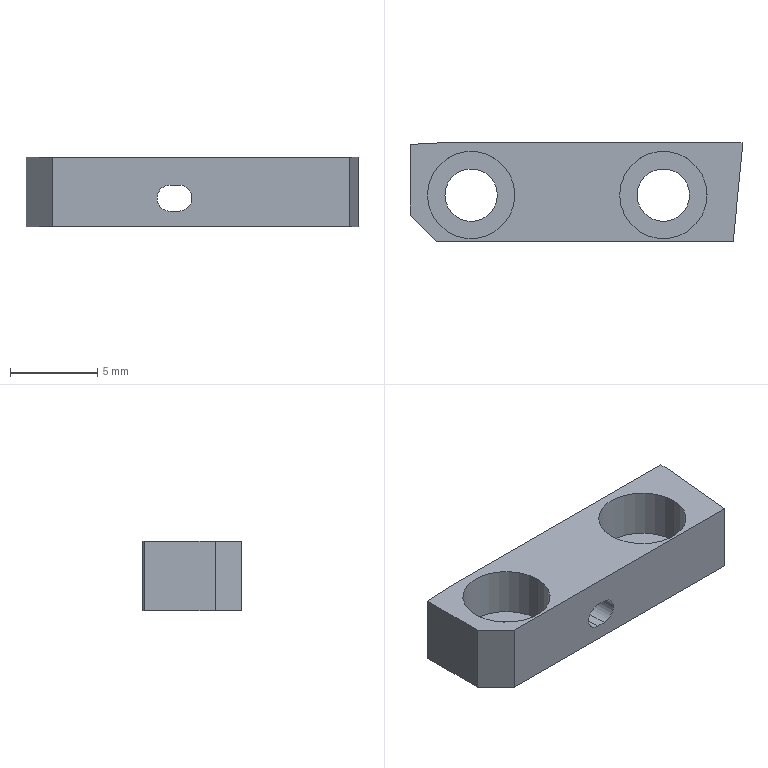Part | NX | 1 solid | 24 faces | box 19 x 5.65 x 4 mm | volume 278.189 mm3 | plane 13 | cylinder 11 | commonest cylinder face diameters 3 x4 5 x4 1.5 x3
STEP:
#1=CARTESIAN_POINT('',(19.,5.15,4.));
#2=VERTEX_POINT('',#1);
#3=CARTESIAN_POINT('',(18.5,0.,4.));
#4=VERTEX_POINT('',#3);
#5=CARTESIAN_POINT('',(18.5,0.,4.));
#6=DIRECTION('',(-0.09663,-0.9953,0.));
#7=VECTOR('',#6,1000.);
#8=LINE('',#5,#7);
#9=EDGE_CURVE('',#2,#4,#8,.T.);
#10=ORIENTED_EDGE('',*,*,#9,.F.);
#11=CARTESIAN_POINT('',(19.,5.65,4.));
#12=VERTEX_POINT('',#11);
#13=CARTESIAN_POINT('',(19.,0.,4.));
#14=DIRECTION('',(0.,1.,0.));
#15=VECTOR('',#14,1000.);
#16=LINE('',#13,#15);
#17=EDGE_CURVE('',#2,#12,#16,.T.);
#18=ORIENTED_EDGE('',*,*,#17,.T.);
#19=CARTESIAN_POINT('',(2.,5.65,4.));
#20=VERTEX_POINT('',#19);
#21=CARTESIAN_POINT('',(0.,5.65,4.));
#22=DIRECTION('',(-1.,0.,0.));
#23=VECTOR('',#22,1000.);
#24=LINE('',#21,#23);
#25=EDGE_CURVE('',#12,#20,#24,.T.);
#26=ORIENTED_EDGE('',*,*,#25,.T.);
#27=CARTESIAN_POINT('',(0.,5.545,4.));
#28=VERTEX_POINT('',#27);
#29=CARTESIAN_POINT('',(0.,5.545,4.));
#30=DIRECTION('',(-0.9986,-0.05234,0.));
#31=VECTOR('',#30,1000.);
#32=LINE('',#29,#31);
#33=EDGE_CURVE('',#20,#28,#32,.T.);
#34=ORIENTED_EDGE('',*,*,#33,.T.);
#35=CARTESIAN_POINT('',(0.,1.5,4.));
#36=VERTEX_POINT('',#35);
#37=CARTESIAN_POINT('',(0.,0.,4.));
#38=DIRECTION('',(0.,1.,0.));
#39=VECTOR('',#38,1000.);
#40=LINE('',#37,#39);
#41=EDGE_CURVE('',#36,#28,#40,.T.);
#42=ORIENTED_EDGE('',*,*,#41,.F.);
#43=CARTESIAN_POINT('',(1.5,0.,4.));
#44=VERTEX_POINT('',#43);
#45=CARTESIAN_POINT('',(1.5,0.,4.));
#46=DIRECTION('',(-0.7071,0.7071,0.));
#47=VECTOR('',#46,1000.);
#48=LINE('',#45,#47);
#49=EDGE_CURVE('',#44,#36,#48,.T.);
#50=ORIENTED_EDGE('',*,*,#49,.F.);
#51=CARTESIAN_POINT('',(0.,0.,4.));
#52=DIRECTION('',(1.,0.,0.));
#53=VECTOR('',#52,1000.);
#54=LINE('',#51,#53);
#55=EDGE_CURVE('',#44,#4,#54,.T.);
#56=ORIENTED_EDGE('',*,*,#55,.T.);
#57=EDGE_LOOP('',(#10,#18,#26,#34,#42,#50,#56));
#58=FACE_BOUND('',#57,.T.);
#59=CARTESIAN_POINT('',(1.,2.65,4.));
#60=VERTEX_POINT('',#59);
#61=CARTESIAN_POINT('',(6.,2.65,4.));
#62=VERTEX_POINT('',#61);
#63=CARTESIAN_POINT('',(3.5,2.65,4.));
#64=DIRECTION('',(0.,0.,1.));
#65=DIRECTION('',(-1.,0.,0.));
#66=AXIS2_PLACEMENT_3D('',#63,#64,#65);
#67=CIRCLE('',#66,2.5);
#68=EDGE_CURVE('',#60,#62,#67,.T.);
#69=ORIENTED_EDGE('',*,*,#68,.F.);
#70=CARTESIAN_POINT('',(3.5,2.65,4.));
#71=DIRECTION('',(0.,0.,1.));
#72=DIRECTION('',(-1.,0.,0.));
#73=AXIS2_PLACEMENT_3D('',#70,#71,#72);
#74=CIRCLE('',#73,2.5);
#75=EDGE_CURVE('',#62,#60,#74,.T.);
#76=ORIENTED_EDGE('',*,*,#75,.F.);
#77=EDGE_LOOP('',(#69,#76));
#78=FACE_BOUND('',#77,.T.);
#79=CARTESIAN_POINT('',(17.,2.65,4.));
#80=VERTEX_POINT('',#79);
#81=CARTESIAN_POINT('',(12.,2.65,4.));
#82=VERTEX_POINT('',#81);
#83=CARTESIAN_POINT('',(14.5,2.65,4.));
#84=DIRECTION('',(0.,0.,1.));
#85=DIRECTION('',(-1.,0.,0.));
#86=AXIS2_PLACEMENT_3D('',#83,#84,#85);
#87=CIRCLE('',#86,2.5);
#88=EDGE_CURVE('',#80,#82,#87,.T.);
#89=ORIENTED_EDGE('',*,*,#88,.F.);
#90=CARTESIAN_POINT('',(14.5,2.65,4.));
#91=DIRECTION('',(0.,0.,1.));
#92=DIRECTION('',(-1.,0.,0.));
#93=AXIS2_PLACEMENT_3D('',#90,#91,#92);
#94=CIRCLE('',#93,2.5);
#95=EDGE_CURVE('',#82,#80,#94,.T.);
#96=ORIENTED_EDGE('',*,*,#95,.F.);
#97=EDGE_LOOP('',(#89,#96));
#98=FACE_BOUND('',#97,.T.);
#99=CARTESIAN_POINT('',(0.,0.,4.));
#100=DIRECTION('',(0.,0.,1.));
#101=DIRECTION('',(1.,0.,0.));
#102=AXIS2_PLACEMENT_3D('',#99,#100,#101);
#103=PLANE('',#102);
#104=ADVANCED_FACE('',(#58,#78,#98),#103,.T.);
#105=CARTESIAN_POINT('',(1.,2.65,1.2));
#106=VERTEX_POINT('',#105);
#107=CARTESIAN_POINT('',(6.,2.65,1.2));
#108=VERTEX_POINT('',#107);
#109=CARTESIAN_POINT('',(3.5,2.65,1.2));
#110=DIRECTION('',(0.,0.,1.));
#111=DIRECTION('',(-1.,0.,0.));
#112=AXIS2_PLACEMENT_3D('',#109,#110,#111);
#113=CIRCLE('',#112,2.5);
#114=EDGE_CURVE('',#106,#108,#113,.T.);
#115=ORIENTED_EDGE('',*,*,#114,.T.);
#116=CARTESIAN_POINT('',(3.5,2.65,1.2));
#117=DIRECTION('',(0.,0.,1.));
#118=DIRECTION('',(-1.,0.,0.));
#119=AXIS2_PLACEMENT_3D('',#116,#117,#118);
#120=CIRCLE('',#119,2.5);
#121=EDGE_CURVE('',#108,#106,#120,.T.);
#122=ORIENTED_EDGE('',*,*,#121,.T.);
#123=EDGE_LOOP('',(#115,#122));
#124=FACE_BOUND('',#123,.T.);
#125=CARTESIAN_POINT('',(2.,2.65,1.2));
#126=VERTEX_POINT('',#125);
#127=CARTESIAN_POINT('',(5.,2.65,1.2));
#128=VERTEX_POINT('',#127);
#129=CARTESIAN_POINT('',(3.5,2.65,1.2));
#130=DIRECTION('',(0.,0.,1.));
#131=DIRECTION('',(-1.,0.,0.));
#132=AXIS2_PLACEMENT_3D('',#129,#130,#131);
#133=CIRCLE('',#132,1.5);
#134=EDGE_CURVE('',#126,#128,#133,.T.);
#135=ORIENTED_EDGE('',*,*,#134,.F.);
#136=CARTESIAN_POINT('',(3.5,2.65,1.2));
#137=DIRECTION('',(0.,0.,1.));
#138=DIRECTION('',(-1.,0.,0.));
#139=AXIS2_PLACEMENT_3D('',#136,#137,#138);
#140=CIRCLE('',#139,1.5);
#141=EDGE_CURVE('',#128,#126,#140,.T.);
#142=ORIENTED_EDGE('',*,*,#141,.F.);
#143=EDGE_LOOP('',(#135,#142));
#144=FACE_BOUND('',#143,.T.);
#145=CARTESIAN_POINT('',(3.5,2.65,1.2));
#146=DIRECTION('',(0.,0.,1.));
#147=DIRECTION('',(1.,0.,0.));
#148=AXIS2_PLACEMENT_3D('',#145,#146,#147);
#149=PLANE('',#148);
#150=ADVANCED_FACE('',(#124,#144),#149,.T.);
#151=CARTESIAN_POINT('',(1.5,0.,0.));
#152=VERTEX_POINT('',#151);
#153=CARTESIAN_POINT('',(1.5,0.,0.));
#154=DIRECTION('',(0.,0.,1.));
#155=VECTOR('',#154,1000.);
#156=LINE('',#153,#155);
#157=EDGE_CURVE('',#152,#44,#156,.T.);
#158=ORIENTED_EDGE('',*,*,#157,.T.);
#159=ORIENTED_EDGE('',*,*,#49,.T.);
#160=CARTESIAN_POINT('',(0.,1.5,0.));
#161=VERTEX_POINT('',#160);
#162=CARTESIAN_POINT('',(0.,1.5,0.));
#163=DIRECTION('',(0.,0.,1.));
#164=VECTOR('',#163,1000.);
#165=LINE('',#162,#164);
#166=EDGE_CURVE('',#161,#36,#165,.T.);
#167=ORIENTED_EDGE('',*,*,#166,.F.);
#168=CARTESIAN_POINT('',(1.5,0.,0.));
#169=DIRECTION('',(0.7071,-0.7071,0.));
#170=VECTOR('',#169,1000.);
#171=LINE('',#168,#170);
#172=EDGE_CURVE('',#161,#152,#171,.T.);
#173=ORIENTED_EDGE('',*,*,#172,.T.);
#174=EDGE_LOOP('',(#158,#159,#167,#173));
#175=FACE_BOUND('',#174,.T.);
#176=CARTESIAN_POINT('',(1.5,0.,0.));
#177=DIRECTION('',(-0.7071,-0.7071,0.));
#178=DIRECTION('',(-0.7071,0.7071,0.));
#179=AXIS2_PLACEMENT_3D('',#176,#177,#178);
#180=PLANE('',#179);
#181=ADVANCED_FACE('',(#175),#180,.T.);
#182=CARTESIAN_POINT('',(0.,5.545,0.));
#183=VERTEX_POINT('',#182);
#184=CARTESIAN_POINT('',(0.,0.,0.));
#185=DIRECTION('',(0.,-1.,0.));
#186=VECTOR('',#185,1000.);
#187=LINE('',#184,#186);
#188=EDGE_CURVE('',#183,#161,#187,.T.);
#189=ORIENTED_EDGE('',*,*,#188,.T.);
#190=ORIENTED_EDGE('',*,*,#166,.T.);
#191=ORIENTED_EDGE('',*,*,#41,.T.);
#192=CARTESIAN_POINT('',(0.,5.545,0.));
#193=DIRECTION('',(0.,0.,-1.));
#194=VECTOR('',#193,1000.);
#195=LINE('',#192,#194);
#196=EDGE_CURVE('',#28,#183,#195,.T.);
#197=ORIENTED_EDGE('',*,*,#196,.T.);
#198=EDGE_LOOP('',(#189,#190,#191,#197));
#199=FACE_BOUND('',#198,.T.);
#200=CARTESIAN_POINT('',(0.,5.65,0.));
#201=DIRECTION('',(-1.,0.,0.));
#202=DIRECTION('',(0.,0.,1.));
#203=AXIS2_PLACEMENT_3D('',#200,#201,#202);
#204=PLANE('',#203);
#205=ADVANCED_FACE('',(#199),#204,.T.);
#206=ORIENTED_EDGE('',*,*,#196,.F.);
#207=ORIENTED_EDGE('',*,*,#33,.F.);
#208=CARTESIAN_POINT('',(2.,5.65,0.));
#209=VERTEX_POINT('',#208);
#210=CARTESIAN_POINT('',(2.,5.65,0.));
#211=DIRECTION('',(0.,0.,-1.));
#212=VECTOR('',#211,1000.);
#213=LINE('',#210,#212);
#214=EDGE_CURVE('',#20,#209,#213,.T.);
#215=ORIENTED_EDGE('',*,*,#214,.T.);
#216=CARTESIAN_POINT('',(0.,5.545,0.));
#217=DIRECTION('',(-0.9986,-0.05234,0.));
#218=VECTOR('',#217,1000.);
#219=LINE('',#216,#218);
#220=EDGE_CURVE('',#209,#183,#219,.T.);
#221=ORIENTED_EDGE('',*,*,#220,.T.);
#222=EDGE_LOOP('',(#206,#207,#215,#221));
#223=FACE_BOUND('',#222,.T.);
#224=CARTESIAN_POINT('',(0.,5.545,0.));
#225=DIRECTION('',(-0.05234,0.9986,0.));
#226=DIRECTION('',(0.,0.,1.));
#227=AXIS2_PLACEMENT_3D('',#224,#225,#226);
#228=PLANE('',#227);
#229=ADVANCED_FACE('',(#223),#228,.T.);
#230=CARTESIAN_POINT('',(19.,5.15,0.));
#231=VERTEX_POINT('',#230);
#232=CARTESIAN_POINT('',(18.5,0.,0.));
#233=VERTEX_POINT('',#232);
#234=CARTESIAN_POINT('',(18.5,0.,0.));
#235=DIRECTION('',(-0.09663,-0.9953,0.));
#236=VECTOR('',#235,1000.);
#237=LINE('',#234,#236);
#238=EDGE_CURVE('',#231,#233,#237,.T.);
#239=ORIENTED_EDGE('',*,*,#238,.T.);
#240=CARTESIAN_POINT('',(0.,0.,0.));
#241=DIRECTION('',(1.,0.,0.));
#242=VECTOR('',#241,1000.);
#243=LINE('',#240,#242);
#244=EDGE_CURVE('',#152,#233,#243,.T.);
#245=ORIENTED_EDGE('',*,*,#244,.F.);
#246=ORIENTED_EDGE('',*,*,#172,.F.);
#247=ORIENTED_EDGE('',*,*,#188,.F.);
#248=ORIENTED_EDGE('',*,*,#220,.F.);
#249=CARTESIAN_POINT('',(19.,5.65,0.));
#250=VERTEX_POINT('',#249);
#251=CARTESIAN_POINT('',(0.,5.65,0.));
#252=DIRECTION('',(-1.,0.,0.));
#253=VECTOR('',#252,1000.);
#254=LINE('',#251,#253);
#255=EDGE_CURVE('',#250,#209,#254,.T.);
#256=ORIENTED_EDGE('',*,*,#255,.F.);
#257=CARTESIAN_POINT('',(19.,0.,0.));
#258=DIRECTION('',(0.,1.,0.));
#259=VECTOR('',#258,1000.);
#260=LINE('',#257,#259);
#261=EDGE_CURVE('',#231,#250,#260,.T.);
#262=ORIENTED_EDGE('',*,*,#261,.F.);
#263=EDGE_LOOP('',(#239,#245,#246,#247,#248,#256,#262));
#264=FACE_BOUND('',#263,.T.);
#265=CARTESIAN_POINT('',(2.,2.65,0.));
#266=VERTEX_POINT('',#265);
#267=CARTESIAN_POINT('',(5.,2.65,0.));
#268=VERTEX_POINT('',#267);
#269=CARTESIAN_POINT('',(3.5,2.65,0.));
#270=DIRECTION('',(0.,0.,1.));
#271=DIRECTION('',(-1.,0.,0.));
#272=AXIS2_PLACEMENT_3D('',#269,#270,#271);
#273=CIRCLE('',#272,1.5);
#274=EDGE_CURVE('',#266,#268,#273,.T.);
#275=ORIENTED_EDGE('',*,*,#274,.T.);
#276=CARTESIAN_POINT('',(3.5,2.65,0.));
#277=DIRECTION('',(0.,0.,1.));
#278=DIRECTION('',(-1.,0.,0.));
#279=AXIS2_PLACEMENT_3D('',#276,#277,#278);
#280=CIRCLE('',#279,1.5);
#281=EDGE_CURVE('',#268,#266,#280,.T.);
#282=ORIENTED_EDGE('',*,*,#281,.T.);
#283=EDGE_LOOP('',(#275,#282));
#284=FACE_BOUND('',#283,.T.);
#285=CARTESIAN_POINT('',(16.,2.65,0.));
#286=VERTEX_POINT('',#285);
#287=CARTESIAN_POINT('',(13.,2.65,0.));
#288=VERTEX_POINT('',#287);
#289=CARTESIAN_POINT('',(14.5,2.65,0.));
#290=DIRECTION('',(0.,0.,1.));
#291=DIRECTION('',(-1.,0.,0.));
#292=AXIS2_PLACEMENT_3D('',#289,#290,#291);
#293=CIRCLE('',#292,1.5);
#294=EDGE_CURVE('',#286,#288,#293,.T.);
#295=ORIENTED_EDGE('',*,*,#294,.T.);
#296=CARTESIAN_POINT('',(14.5,2.65,0.));
#297=DIRECTION('',(0.,0.,1.));
#298=DIRECTION('',(-1.,0.,0.));
#299=AXIS2_PLACEMENT_3D('',#296,#297,#298);
#300=CIRCLE('',#299,1.5);
#301=EDGE_CURVE('',#288,#286,#300,.T.);
#302=ORIENTED_EDGE('',*,*,#301,.T.);
#303=EDGE_LOOP('',(#295,#302));
#304=FACE_BOUND('',#303,.T.);
#305=CARTESIAN_POINT('',(0.,0.,0.));
#306=DIRECTION('',(0.,0.,1.));
#307=DIRECTION('',(1.,0.,0.));
#308=AXIS2_PLACEMENT_3D('',#305,#306,#307);
#309=PLANE('',#308);
#310=ADVANCED_FACE('',(#264,#284,#304),#309,.F.);
#311=ORIENTED_EDGE('',*,*,#261,.T.);
#312=CARTESIAN_POINT('',(19.,5.65,0.));
#313=DIRECTION('',(0.,0.,1.));
#314=VECTOR('',#313,1000.);
#315=LINE('',#312,#314);
#316=EDGE_CURVE('',#250,#12,#315,.T.);
#317=ORIENTED_EDGE('',*,*,#316,.T.);
#318=ORIENTED_EDGE('',*,*,#17,.F.);
#319=CARTESIAN_POINT('',(19.,5.15,0.));
#320=DIRECTION('',(0.,0.,1.));
#321=VECTOR('',#320,1000.);
#322=LINE('',#319,#321);
#323=EDGE_CURVE('',#231,#2,#322,.T.);
#324=ORIENTED_EDGE('',*,*,#323,.F.);
#325=EDGE_LOOP('',(#311,#317,#318,#324));
#326=FACE_BOUND('',#325,.T.);
#327=CARTESIAN_POINT('',(19.,0.,0.));
#328=DIRECTION('',(1.,0.,0.));
#329=DIRECTION('',(0.,1.,0.));
#330=AXIS2_PLACEMENT_3D('',#327,#328,#329);
#331=PLANE('',#330);
#332=ADVANCED_FACE('',(#326),#331,.T.);
#333=ORIENTED_EDGE('',*,*,#238,.F.);
#334=ORIENTED_EDGE('',*,*,#323,.T.);
#335=ORIENTED_EDGE('',*,*,#9,.T.);
#336=CARTESIAN_POINT('',(18.5,0.,0.));
#337=DIRECTION('',(0.,0.,-1.));
#338=VECTOR('',#337,1000.);
#339=LINE('',#336,#338);
#340=EDGE_CURVE('',#4,#233,#339,.T.);
#341=ORIENTED_EDGE('',*,*,#340,.T.);
#342=EDGE_LOOP('',(#333,#334,#335,#341));
#343=FACE_BOUND('',#342,.T.);
#344=CARTESIAN_POINT('',(18.5,0.,-0.45));
#345=DIRECTION('',(-0.9953,0.09663,0.));
#346=DIRECTION('',(0.,0.,1.));
#347=AXIS2_PLACEMENT_3D('',#344,#345,#346);
#348=PLANE('',#347);
#349=ADVANCED_FACE('',(#343),#348,.F.);
#350=ORIENTED_EDGE('',*,*,#114,.F.);
#351=CARTESIAN_POINT('',(1.,2.65,-0.775));
#352=DIRECTION('',(0.,0.,1.));
#353=VECTOR('',#352,1000.);
#354=LINE('',#351,#353);
#355=EDGE_CURVE('',#60,#106,#354,.F.);
#356=ORIENTED_EDGE('',*,*,#355,.F.);
#357=ORIENTED_EDGE('',*,*,#68,.T.);
#358=CARTESIAN_POINT('',(6.,2.65,-0.775));
#359=DIRECTION('',(0.,0.,1.));
#360=VECTOR('',#359,1000.);
#361=LINE('',#358,#360);
#362=EDGE_CURVE('',#62,#108,#361,.F.);
#363=ORIENTED_EDGE('',*,*,#362,.T.);
#364=EDGE_LOOP('',(#350,#356,#357,#363));
#365=FACE_BOUND('',#364,.T.);
#366=CARTESIAN_POINT('',(3.5,2.65,-0.775));
#367=DIRECTION('',(0.,0.,1.));
#368=DIRECTION('',(-1.,0.,0.));
#369=AXIS2_PLACEMENT_3D('',#366,#367,#368);
#370=CYLINDRICAL_SURFACE('',#369,2.5);
#371=ADVANCED_FACE('',(#365),#370,.F.);
#372=CARTESIAN_POINT('',(17.,2.65,1.2));
#373=VERTEX_POINT('',#372);
#374=CARTESIAN_POINT('',(12.,2.65,1.2));
#375=VERTEX_POINT('',#374);
#376=CARTESIAN_POINT('',(14.5,2.65,1.2));
#377=DIRECTION('',(0.,0.,1.));
#378=DIRECTION('',(-1.,0.,0.));
#379=AXIS2_PLACEMENT_3D('',#376,#377,#378);
#380=CIRCLE('',#379,2.5);
#381=EDGE_CURVE('',#373,#375,#380,.T.);
#382=ORIENTED_EDGE('',*,*,#381,.T.);
#383=CARTESIAN_POINT('',(14.5,2.65,1.2));
#384=DIRECTION('',(0.,0.,1.));
#385=DIRECTION('',(-1.,0.,0.));
#386=AXIS2_PLACEMENT_3D('',#383,#384,#385);
#387=CIRCLE('',#386,2.5);
#388=EDGE_CURVE('',#375,#373,#387,.T.);
#389=ORIENTED_EDGE('',*,*,#388,.T.);
#390=EDGE_LOOP('',(#382,#389));
#391=FACE_BOUND('',#390,.T.);
#392=CARTESIAN_POINT('',(13.,2.65,1.2));
#393=VERTEX_POINT('',#392);
#394=CARTESIAN_POINT('',(16.,2.65,1.2));
#395=VERTEX_POINT('',#394);
#396=CARTESIAN_POINT('',(14.5,2.65,1.2));
#397=DIRECTION('',(0.,0.,1.));
#398=DIRECTION('',(-1.,0.,0.));
#399=AXIS2_PLACEMENT_3D('',#396,#397,#398);
#400=CIRCLE('',#399,1.5);
#401=EDGE_CURVE('',#393,#395,#400,.T.);
#402=ORIENTED_EDGE('',*,*,#401,.F.);
#403=CARTESIAN_POINT('',(14.5,2.65,1.2));
#404=DIRECTION('',(0.,0.,1.));
#405=DIRECTION('',(-1.,0.,0.));
#406=AXIS2_PLACEMENT_3D('',#403,#404,#405);
#407=CIRCLE('',#406,1.5);
#408=EDGE_CURVE('',#395,#393,#407,.T.);
#409=ORIENTED_EDGE('',*,*,#408,.F.);
#410=EDGE_LOOP('',(#402,#409));
#411=FACE_BOUND('',#410,.T.);
#412=CARTESIAN_POINT('',(14.5,2.65,1.2));
#413=DIRECTION('',(0.,0.,1.));
#414=DIRECTION('',(1.,0.,0.));
#415=AXIS2_PLACEMENT_3D('',#412,#413,#414);
#416=PLANE('',#415);
#417=ADVANCED_FACE('',(#391,#411),#416,.T.);
#418=ORIENTED_EDGE('',*,*,#340,.F.);
#419=ORIENTED_EDGE('',*,*,#55,.F.);
#420=ORIENTED_EDGE('',*,*,#157,.F.);
#421=ORIENTED_EDGE('',*,*,#244,.T.);
#422=EDGE_LOOP('',(#418,#419,#420,#421));
#423=FACE_BOUND('',#422,.T.);
#424=CARTESIAN_POINT('',(8.25,0.,2.4));
#425=VERTEX_POINT('',#424);
#426=CARTESIAN_POINT('',(8.75,0.,2.4));
#427=VERTEX_POINT('',#426);
#428=CARTESIAN_POINT('',(0.,0.,2.4));
#429=DIRECTION('',(1.,0.,0.));
#430=VECTOR('',#429,1000.);
#431=LINE('',#428,#430);
#432=EDGE_CURVE('',#425,#427,#431,.T.);
#433=ORIENTED_EDGE('',*,*,#432,.T.);
#434=CARTESIAN_POINT('',(8.75,0.,0.9));
#435=VERTEX_POINT('',#434);
#436=CARTESIAN_POINT('',(8.75,0.,1.65));
#437=DIRECTION('',(0.,1.,0.));
#438=DIRECTION('',(-1.,0.,0.));
#439=AXIS2_PLACEMENT_3D('',#436,#437,#438);
#440=CIRCLE('',#439,0.75);
#441=EDGE_CURVE('',#427,#435,#440,.T.);
#442=ORIENTED_EDGE('',*,*,#441,.T.);
#443=CARTESIAN_POINT('',(8.25,0.,0.9));
#444=VERTEX_POINT('',#443);
#445=CARTESIAN_POINT('',(0.,0.,0.9));
#446=DIRECTION('',(-1.,0.,0.));
#447=VECTOR('',#446,1000.);
#448=LINE('',#445,#447);
#449=EDGE_CURVE('',#435,#444,#448,.T.);
#450=ORIENTED_EDGE('',*,*,#449,.T.);
#451=CARTESIAN_POINT('',(7.5,0.,1.65));
#452=VERTEX_POINT('',#451);
#453=CARTESIAN_POINT('',(8.25,0.,1.65));
#454=DIRECTION('',(0.,1.,0.));
#455=DIRECTION('',(-1.,0.,0.));
#456=AXIS2_PLACEMENT_3D('',#453,#454,#455);
#457=CIRCLE('',#456,0.75);
#458=EDGE_CURVE('',#444,#452,#457,.T.);
#459=ORIENTED_EDGE('',*,*,#458,.T.);
#460=CARTESIAN_POINT('',(8.25,0.,1.65));
#461=DIRECTION('',(0.,1.,0.));
#462=DIRECTION('',(-1.,0.,0.));
#463=AXIS2_PLACEMENT_3D('',#460,#461,#462);
#464=CIRCLE('',#463,0.75);
#465=EDGE_CURVE('',#452,#425,#464,.T.);
#466=ORIENTED_EDGE('',*,*,#465,.T.);
#467=EDGE_LOOP('',(#433,#442,#450,#459,#466));
#468=FACE_BOUND('',#467,.T.);
#469=CARTESIAN_POINT('',(0.,0.,0.));
#470=DIRECTION('',(0.,-1.,0.));
#471=DIRECTION('',(0.,0.,-1.));
#472=AXIS2_PLACEMENT_3D('',#469,#470,#471);
#473=PLANE('',#472);
#474=ADVANCED_FACE('',(#423,#468),#473,.T.);
#475=ORIENTED_EDGE('',*,*,#274,.F.);
#476=CARTESIAN_POINT('',(2.,2.65,-0.775));
#477=DIRECTION('',(0.,0.,1.));
#478=VECTOR('',#477,1000.);
#479=LINE('',#476,#478);
#480=EDGE_CURVE('',#126,#266,#479,.F.);
#481=ORIENTED_EDGE('',*,*,#480,.F.);
#482=ORIENTED_EDGE('',*,*,#134,.T.);
#483=CARTESIAN_POINT('',(5.,2.65,-0.775));
#484=DIRECTION('',(0.,0.,1.));
#485=VECTOR('',#484,1000.);
#486=LINE('',#483,#485);
#487=EDGE_CURVE('',#128,#268,#486,.F.);
#488=ORIENTED_EDGE('',*,*,#487,.T.);
#489=EDGE_LOOP('',(#475,#481,#482,#488));
#490=FACE_BOUND('',#489,.T.);
#491=CARTESIAN_POINT('',(3.5,2.65,-0.775));
#492=DIRECTION('',(0.,0.,1.));
#493=DIRECTION('',(-1.,0.,0.));
#494=AXIS2_PLACEMENT_3D('',#491,#492,#493);
#495=CYLINDRICAL_SURFACE('',#494,1.5);
#496=ADVANCED_FACE('',(#490),#495,.F.);
#497=ORIENTED_EDGE('',*,*,#294,.F.);
#498=CARTESIAN_POINT('',(16.,2.65,-0.775));
#499=DIRECTION('',(0.,0.,1.));
#500=VECTOR('',#499,1000.);
#501=LINE('',#498,#500);
#502=EDGE_CURVE('',#286,#395,#501,.T.);
#503=ORIENTED_EDGE('',*,*,#502,.T.);
#504=ORIENTED_EDGE('',*,*,#408,.T.);
#505=CARTESIAN_POINT('',(13.,2.65,-0.775));
#506=DIRECTION('',(0.,0.,1.));
#507=VECTOR('',#506,1000.);
#508=LINE('',#505,#507);
#509=EDGE_CURVE('',#288,#393,#508,.T.);
#510=ORIENTED_EDGE('',*,*,#509,.F.);
#511=EDGE_LOOP('',(#497,#503,#504,#510));
#512=FACE_BOUND('',#511,.T.);
#513=CARTESIAN_POINT('',(14.5,2.65,-0.775));
#514=DIRECTION('',(0.,0.,1.));
#515=DIRECTION('',(-1.,0.,0.));
#516=AXIS2_PLACEMENT_3D('',#513,#514,#515);
#517=CYLINDRICAL_SURFACE('',#516,1.5);
#518=ADVANCED_FACE('',(#512),#517,.F.);
#519=ORIENTED_EDGE('',*,*,#381,.F.);
#520=CARTESIAN_POINT('',(17.,2.65,-0.775));
#521=DIRECTION('',(0.,0.,1.));
#522=VECTOR('',#521,1000.);
#523=LINE('',#520,#522);
#524=EDGE_CURVE('',#80,#373,#523,.F.);
#525=ORIENTED_EDGE('',*,*,#524,.F.);
#526=ORIENTED_EDGE('',*,*,#88,.T.);
#527=CARTESIAN_POINT('',(12.,2.65,-0.775));
#528=DIRECTION('',(0.,0.,1.));
#529=VECTOR('',#528,1000.);
#530=LINE('',#527,#529);
#531=EDGE_CURVE('',#82,#375,#530,.F.);
#532=ORIENTED_EDGE('',*,*,#531,.T.);
#533=EDGE_LOOP('',(#519,#525,#526,#532));
#534=FACE_BOUND('',#533,.T.);
#535=CARTESIAN_POINT('',(14.5,2.65,-0.775));
#536=DIRECTION('',(0.,0.,1.));
#537=DIRECTION('',(-1.,0.,0.));
#538=AXIS2_PLACEMENT_3D('',#535,#536,#537);
#539=CYLINDRICAL_SURFACE('',#538,2.5);
#540=ADVANCED_FACE('',(#534),#539,.F.);
#541=ORIENTED_EDGE('',*,*,#255,.T.);
#542=ORIENTED_EDGE('',*,*,#214,.F.);
#543=ORIENTED_EDGE('',*,*,#25,.F.);
#544=ORIENTED_EDGE('',*,*,#316,.F.);
#545=EDGE_LOOP('',(#541,#542,#543,#544));
#546=FACE_BOUND('',#545,.T.);
#547=CARTESIAN_POINT('',(8.25,5.65,0.9));
#548=VERTEX_POINT('',#547);
#549=CARTESIAN_POINT('',(8.75,5.65,0.9));
#550=VERTEX_POINT('',#549);
#551=CARTESIAN_POINT('',(0.,5.65,0.9));
#552=DIRECTION('',(1.,0.,0.));
#553=VECTOR('',#552,1000.);
#554=LINE('',#551,#553);
#555=EDGE_CURVE('',#548,#550,#554,.T.);
#556=ORIENTED_EDGE('',*,*,#555,.T.);
#557=CARTESIAN_POINT('',(8.75,5.65,2.4));
#558=VERTEX_POINT('',#557);
#559=CARTESIAN_POINT('',(8.75,5.65,1.65));
#560=DIRECTION('',(0.,1.,0.));
#561=DIRECTION('',(-1.,0.,0.));
#562=AXIS2_PLACEMENT_3D('',#559,#560,#561);
#563=CIRCLE('',#562,0.75);
#564=EDGE_CURVE('',#558,#550,#563,.T.);
#565=ORIENTED_EDGE('',*,*,#564,.F.);
#566=CARTESIAN_POINT('',(8.25,5.65,2.4));
#567=VERTEX_POINT('',#566);
#568=CARTESIAN_POINT('',(0.,5.65,2.4));
#569=DIRECTION('',(-1.,0.,0.));
#570=VECTOR('',#569,1000.);
#571=LINE('',#568,#570);
#572=EDGE_CURVE('',#558,#567,#571,.T.);
#573=ORIENTED_EDGE('',*,*,#572,.T.);
#574=CARTESIAN_POINT('',(7.5,5.65,1.65));
#575=VERTEX_POINT('',#574);
#576=CARTESIAN_POINT('',(8.25,5.65,1.65));
#577=DIRECTION('',(0.,1.,0.));
#578=DIRECTION('',(-1.,0.,0.));
#579=AXIS2_PLACEMENT_3D('',#576,#577,#578);
#580=CIRCLE('',#579,0.75);
#581=EDGE_CURVE('',#575,#567,#580,.T.);
#582=ORIENTED_EDGE('',*,*,#581,.F.);
#583=CARTESIAN_POINT('',(8.25,5.65,1.65));
#584=DIRECTION('',(0.,1.,0.));
#585=DIRECTION('',(-1.,0.,0.));
#586=AXIS2_PLACEMENT_3D('',#583,#584,#585);
#587=CIRCLE('',#586,0.75);
#588=EDGE_CURVE('',#548,#575,#587,.T.);
#589=ORIENTED_EDGE('',*,*,#588,.F.);
#590=EDGE_LOOP('',(#556,#565,#573,#582,#589));
#591=FACE_BOUND('',#590,.T.);
#592=CARTESIAN_POINT('',(19.,5.65,0.));
#593=DIRECTION('',(0.,1.,0.));
#594=DIRECTION('',(1.,0.,0.));
#595=AXIS2_PLACEMENT_3D('',#592,#593,#594);
#596=PLANE('',#595);
#597=ADVANCED_FACE('',(#546,#591),#596,.T.);
#598=CARTESIAN_POINT('',(7.5,-0.565,1.65));
#599=DIRECTION('',(0.,1.,0.));
#600=VECTOR('',#599,1000.);
#601=LINE('',#598,#600);
#602=EDGE_CURVE('',#452,#575,#601,.T.);
#603=ORIENTED_EDGE('',*,*,#602,.F.);
#604=ORIENTED_EDGE('',*,*,#458,.F.);
#605=CARTESIAN_POINT('',(8.25,-0.565,0.9));
#606=DIRECTION('',(0.,1.,0.));
#607=VECTOR('',#606,1000.);
#608=LINE('',#605,#607);
#609=EDGE_CURVE('',#444,#548,#608,.T.);
#610=ORIENTED_EDGE('',*,*,#609,.T.);
#611=ORIENTED_EDGE('',*,*,#588,.T.);
#612=EDGE_LOOP('',(#603,#604,#610,#611));
#613=FACE_BOUND('',#612,.T.);
#614=CARTESIAN_POINT('',(8.25,-0.565,1.65));
#615=DIRECTION('',(0.,1.,0.));
#616=DIRECTION('',(-1.,0.,0.));
#617=AXIS2_PLACEMENT_3D('',#614,#615,#616);
#618=CYLINDRICAL_SURFACE('',#617,0.75);
#619=ADVANCED_FACE('',(#613),#618,.F.);
#620=ORIENTED_EDGE('',*,*,#441,.F.);
#621=CARTESIAN_POINT('',(8.75,-0.565,2.4));
#622=DIRECTION('',(0.,1.,0.));
#623=VECTOR('',#622,1000.);
#624=LINE('',#621,#623);
#625=EDGE_CURVE('',#427,#558,#624,.T.);
#626=ORIENTED_EDGE('',*,*,#625,.T.);
#627=ORIENTED_EDGE('',*,*,#564,.T.);
#628=CARTESIAN_POINT('',(8.75,-0.565,0.9));
#629=DIRECTION('',(0.,1.,0.));
#630=VECTOR('',#629,1000.);
#631=LINE('',#628,#630);
#632=EDGE_CURVE('',#435,#550,#631,.T.);
#633=ORIENTED_EDGE('',*,*,#632,.F.);
#634=EDGE_LOOP('',(#620,#626,#627,#633));
#635=FACE_BOUND('',#634,.T.);
#636=CARTESIAN_POINT('',(8.75,-0.565,1.65));
#637=DIRECTION('',(0.,1.,0.));
#638=DIRECTION('',(-1.,0.,0.));
#639=AXIS2_PLACEMENT_3D('',#636,#637,#638);
#640=CYLINDRICAL_SURFACE('',#639,0.75);
#641=ADVANCED_FACE('',(#635),#640,.F.);
#642=ORIENTED_EDGE('',*,*,#555,.F.);
#643=ORIENTED_EDGE('',*,*,#609,.F.);
#644=ORIENTED_EDGE('',*,*,#449,.F.);
#645=ORIENTED_EDGE('',*,*,#632,.T.);
#646=EDGE_LOOP('',(#642,#643,#644,#645));
#647=FACE_BOUND('',#646,.T.);
#648=CARTESIAN_POINT('',(8.25,-0.565,0.9));
#649=DIRECTION('',(0.,0.,-1.));
#650=DIRECTION('',(0.,-1.,0.));
#651=AXIS2_PLACEMENT_3D('',#648,#649,#650);
#652=PLANE('',#651);
#653=ADVANCED_FACE('',(#647),#652,.F.);
#654=ORIENTED_EDGE('',*,*,#432,.F.);
#655=CARTESIAN_POINT('',(8.25,-0.565,2.4));
#656=DIRECTION('',(0.,1.,0.));
#657=VECTOR('',#656,1000.);
#658=LINE('',#655,#657);
#659=EDGE_CURVE('',#425,#567,#658,.T.);
#660=ORIENTED_EDGE('',*,*,#659,.T.);
#661=ORIENTED_EDGE('',*,*,#572,.F.);
#662=ORIENTED_EDGE('',*,*,#625,.F.);
#663=EDGE_LOOP('',(#654,#660,#661,#662));
#664=FACE_BOUND('',#663,.T.);
#665=CARTESIAN_POINT('',(8.75,-0.565,2.4));
#666=DIRECTION('',(0.,0.,1.));
#667=DIRECTION('',(1.,0.,0.));
#668=AXIS2_PLACEMENT_3D('',#665,#666,#667);
#669=PLANE('',#668);
#670=ADVANCED_FACE('',(#664),#669,.F.);
#671=ORIENTED_EDGE('',*,*,#480,.T.);
#672=ORIENTED_EDGE('',*,*,#281,.F.);
#673=ORIENTED_EDGE('',*,*,#487,.F.);
#674=ORIENTED_EDGE('',*,*,#141,.T.);
#675=EDGE_LOOP('',(#671,#672,#673,#674));
#676=FACE_BOUND('',#675,.T.);
#677=CARTESIAN_POINT('',(3.5,2.65,-0.775));
#678=DIRECTION('',(0.,0.,1.));
#679=DIRECTION('',(-1.,0.,0.));
#680=AXIS2_PLACEMENT_3D('',#677,#678,#679);
#681=CYLINDRICAL_SURFACE('',#680,1.5);
#682=ADVANCED_FACE('',(#676),#681,.F.);
#683=ORIENTED_EDGE('',*,*,#531,.F.);
#684=ORIENTED_EDGE('',*,*,#95,.T.);
#685=ORIENTED_EDGE('',*,*,#524,.T.);
#686=ORIENTED_EDGE('',*,*,#388,.F.);
#687=EDGE_LOOP('',(#683,#684,#685,#686));
#688=FACE_BOUND('',#687,.T.);
#689=CARTESIAN_POINT('',(14.5,2.65,-0.775));
#690=DIRECTION('',(0.,0.,1.));
#691=DIRECTION('',(-1.,0.,0.));
#692=AXIS2_PLACEMENT_3D('',#689,#690,#691);
#693=CYLINDRICAL_SURFACE('',#692,2.5);
#694=ADVANCED_FACE('',(#688),#693,.F.);
#695=ORIENTED_EDGE('',*,*,#401,.T.);
#696=ORIENTED_EDGE('',*,*,#502,.F.);
#697=ORIENTED_EDGE('',*,*,#301,.F.);
#698=ORIENTED_EDGE('',*,*,#509,.T.);
#699=EDGE_LOOP('',(#695,#696,#697,#698));
#700=FACE_BOUND('',#699,.T.);
#701=CARTESIAN_POINT('',(14.5,2.65,-0.775));
#702=DIRECTION('',(0.,0.,1.));
#703=DIRECTION('',(-1.,0.,0.));
#704=AXIS2_PLACEMENT_3D('',#701,#702,#703);
#705=CYLINDRICAL_SURFACE('',#704,1.5);
#706=ADVANCED_FACE('',(#700),#705,.F.);
#707=ORIENTED_EDGE('',*,*,#355,.T.);
#708=ORIENTED_EDGE('',*,*,#121,.F.);
#709=ORIENTED_EDGE('',*,*,#362,.F.);
#710=ORIENTED_EDGE('',*,*,#75,.T.);
#711=EDGE_LOOP('',(#707,#708,#709,#710));
#712=FACE_BOUND('',#711,.T.);
#713=CARTESIAN_POINT('',(3.5,2.65,-0.775));
#714=DIRECTION('',(0.,0.,1.));
#715=DIRECTION('',(-1.,0.,0.));
#716=AXIS2_PLACEMENT_3D('',#713,#714,#715);
#717=CYLINDRICAL_SURFACE('',#716,2.5);
#718=ADVANCED_FACE('',(#712),#717,.F.);
#719=ORIENTED_EDGE('',*,*,#465,.F.);
#720=ORIENTED_EDGE('',*,*,#602,.T.);
#721=ORIENTED_EDGE('',*,*,#581,.T.);
#722=ORIENTED_EDGE('',*,*,#659,.F.);
#723=EDGE_LOOP('',(#719,#720,#721,#722));
#724=FACE_BOUND('',#723,.T.);
#725=CARTESIAN_POINT('',(8.25,-0.565,1.65));
#726=DIRECTION('',(0.,1.,0.));
#727=DIRECTION('',(-1.,0.,0.));
#728=AXIS2_PLACEMENT_3D('',#725,#726,#727);
#729=CYLINDRICAL_SURFACE('',#728,0.75);
#730=ADVANCED_FACE('',(#724),#729,.F.);
#731=CLOSED_SHELL('',(#104,#150,#181,#205,#229,#310,#332,#349,#371,#417,#474,#496,#518,#540,#597,#619,#641,#653,#670,#682,#694,#706,#718,#730));
#732=MANIFOLD_SOLID_BREP('',#731);
#733=(LENGTH_UNIT()NAMED_UNIT(*)SI_UNIT(.MILLI.,.METRE.));
#734=UNCERTAINTY_MEASURE_WITH_UNIT(LENGTH_MEASURE(0.00001),#733,'','');
#735=(NAMED_UNIT(*)PLANE_ANGLE_UNIT()SI_UNIT($,.RADIAN.));
#736=(NAMED_UNIT(*)SI_UNIT($,.STERADIAN.)SOLID_ANGLE_UNIT());
#737=(GEOMETRIC_REPRESENTATION_CONTEXT(3)GLOBAL_UNCERTAINTY_ASSIGNED_CONTEXT((#734))GLOBAL_UNIT_ASSIGNED_CONTEXT((#733,#735,#736))REPRESENTATION_CONTEXT('',''));
#738=ADVANCED_BREP_SHAPE_REPRESENTATION('',(#732),#737);